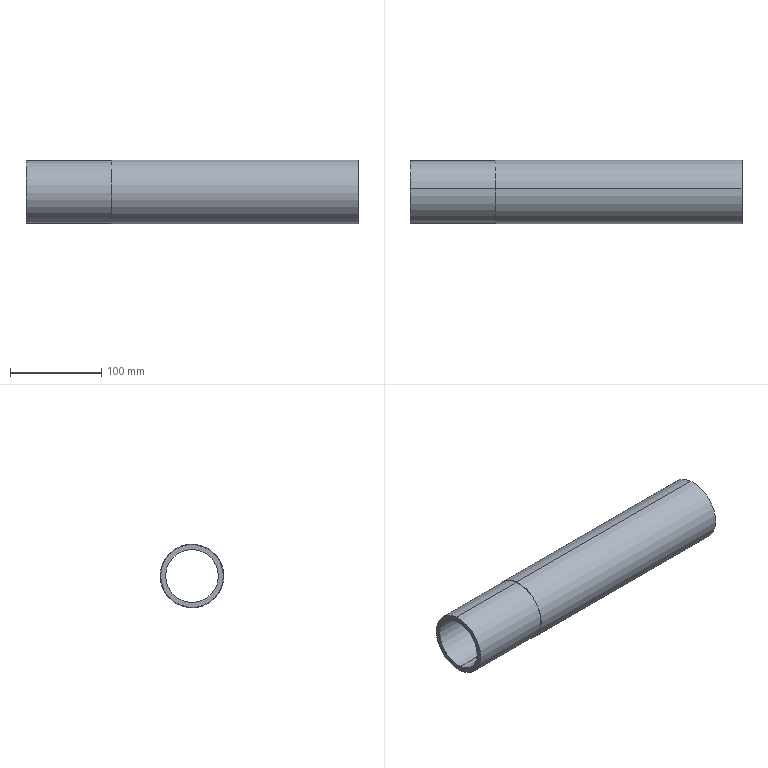Part | NX | features BREP 1 | 1 solid | 9 faces | box 364.46 x 70 x 70 mm | volume 429462 mm3 | cylinder 6 | plane 3 | commonest cylinder face diameters 58 x2 69 x2 70 x2
STEP:
#1=CARTESIAN_POINT('',(131.205,-2.874,-28.857));
#2=VERTEX_POINT('',#1);
#3=CARTESIAN_POINT('',(131.205,2.874,28.857));
#4=VERTEX_POINT('',#3);
#5=CARTESIAN_POINT('',(131.205,0.,0.));
#6=DIRECTION('',(-1.,0.,0.));
#7=DIRECTION('',(0.,0.09911,0.9951));
#8=AXIS2_PLACEMENT_3D('',#5,#6,#7);
#9=CIRCLE('',#8,29.);
#10=EDGE_CURVE('',#2,#4,#9,.T.);
#11=ORIENTED_EDGE('',*,*,#10,.T.);
#12=CARTESIAN_POINT('',(495.665,2.874,28.857));
#13=VERTEX_POINT('',#12);
#14=CARTESIAN_POINT('',(602.745,2.874,28.857));
#15=DIRECTION('',(1.,0.,0.));
#16=VECTOR('',#15,1000.);
#17=LINE('',#14,#16);
#18=EDGE_CURVE('',#13,#4,#17,.F.);
#19=ORIENTED_EDGE('',*,*,#18,.F.);
#20=CARTESIAN_POINT('',(495.665,-2.874,-28.857));
#21=VERTEX_POINT('',#20);
#22=CARTESIAN_POINT('',(495.665,0.,0.));
#23=DIRECTION('',(1.,0.,0.));
#24=DIRECTION('',(0.,0.,-1.));
#25=AXIS2_PLACEMENT_3D('',#22,#23,#24);
#26=CIRCLE('',#25,29.);
#27=EDGE_CURVE('',#13,#21,#26,.T.);
#28=ORIENTED_EDGE('',*,*,#27,.T.);
#29=CARTESIAN_POINT('',(602.745,-2.874,-28.857));
#30=DIRECTION('',(1.,0.,0.));
#31=VECTOR('',#30,1000.);
#32=LINE('',#29,#31);
#33=EDGE_CURVE('',#21,#2,#32,.F.);
#34=ORIENTED_EDGE('',*,*,#33,.T.);
#35=EDGE_LOOP('',(#11,#19,#28,#34));
#36=FACE_BOUND('',#35,.T.);
#37=CARTESIAN_POINT('',(602.745,0.,0.));
#38=DIRECTION('',(1.,0.,0.));
#39=DIRECTION('',(0.,0.09911,0.9951));
#40=AXIS2_PLACEMENT_3D('',#37,#38,#39);
#41=CYLINDRICAL_SURFACE('',#40,29.);
#42=ADVANCED_FACE('',(#36),#41,.F.);
#43=CARTESIAN_POINT('',(131.205,3.419,34.33));
#44=VERTEX_POINT('',#43);
#45=CARTESIAN_POINT('',(131.205,-3.419,-34.33));
#46=VERTEX_POINT('',#45);
#47=CARTESIAN_POINT('',(131.205,0.,0.));
#48=DIRECTION('',(-1.,0.,0.));
#49=DIRECTION('',(0.,0.09911,0.9951));
#50=AXIS2_PLACEMENT_3D('',#47,#48,#49);
#51=CIRCLE('',#50,34.5);
#52=EDGE_CURVE('',#44,#46,#51,.T.);
#53=ORIENTED_EDGE('',*,*,#52,.F.);
#54=CARTESIAN_POINT('',(224.745,3.419,34.33));
#55=VERTEX_POINT('',#54);
#56=CARTESIAN_POINT('',(131.205,3.419,34.33));
#57=DIRECTION('',(1.,0.,0.));
#58=VECTOR('',#57,1000.);
#59=LINE('',#56,#58);
#60=EDGE_CURVE('',#55,#44,#59,.F.);
#61=ORIENTED_EDGE('',*,*,#60,.F.);
#62=CARTESIAN_POINT('',(224.745,-3.419,-34.33));
#63=VERTEX_POINT('',#62);
#64=CARTESIAN_POINT('',(224.745,0.,0.));
#65=DIRECTION('',(-1.,0.,0.));
#66=DIRECTION('',(0.,0.09911,0.9951));
#67=AXIS2_PLACEMENT_3D('',#64,#65,#66);
#68=CIRCLE('',#67,34.5);
#69=EDGE_CURVE('',#55,#63,#68,.T.);
#70=ORIENTED_EDGE('',*,*,#69,.T.);
#71=CARTESIAN_POINT('',(131.205,-3.419,-34.33));
#72=DIRECTION('',(1.,0.,0.));
#73=VECTOR('',#72,1000.);
#74=LINE('',#71,#73);
#75=EDGE_CURVE('',#63,#46,#74,.F.);
#76=ORIENTED_EDGE('',*,*,#75,.T.);
#77=EDGE_LOOP('',(#53,#61,#70,#76));
#78=FACE_BOUND('',#77,.T.);
#79=CARTESIAN_POINT('',(131.205,0.,0.));
#80=DIRECTION('',(1.,0.,0.));
#81=DIRECTION('',(0.,0.09911,0.9951));
#82=AXIS2_PLACEMENT_3D('',#79,#80,#81);
#83=CYLINDRICAL_SURFACE('',#82,34.5);
#84=ADVANCED_FACE('',(#78),#83,.T.);
#85=CARTESIAN_POINT('',(224.745,-3.469,-34.828));
#86=VERTEX_POINT('',#85);
#87=CARTESIAN_POINT('',(224.745,3.469,34.828));
#88=VERTEX_POINT('',#87);
#89=CARTESIAN_POINT('',(224.745,0.,0.));
#90=DIRECTION('',(1.,0.,0.));
#91=DIRECTION('',(0.,-0.09911,-0.9951));
#92=AXIS2_PLACEMENT_3D('',#89,#90,#91);
#93=CIRCLE('',#92,35.);
#94=EDGE_CURVE('',#86,#88,#93,.T.);
#95=ORIENTED_EDGE('',*,*,#94,.T.);
#96=CARTESIAN_POINT('',(495.665,3.469,34.828));
#97=VERTEX_POINT('',#96);
#98=CARTESIAN_POINT('',(602.745,3.469,34.828));
#99=DIRECTION('',(1.,0.,0.));
#100=VECTOR('',#99,1000.);
#101=LINE('',#98,#100);
#102=EDGE_CURVE('',#97,#88,#101,.F.);
#103=ORIENTED_EDGE('',*,*,#102,.F.);
#104=CARTESIAN_POINT('',(495.665,-3.469,-34.828));
#105=VERTEX_POINT('',#104);
#106=CARTESIAN_POINT('',(495.665,0.,0.));
#107=DIRECTION('',(-1.,0.,0.));
#108=DIRECTION('',(0.,0.,-1.));
#109=AXIS2_PLACEMENT_3D('',#106,#107,#108);
#110=CIRCLE('',#109,35.);
#111=EDGE_CURVE('',#97,#105,#110,.T.);
#112=ORIENTED_EDGE('',*,*,#111,.T.);
#113=CARTESIAN_POINT('',(602.745,-3.469,-34.828));
#114=DIRECTION('',(1.,0.,0.));
#115=VECTOR('',#114,1000.);
#116=LINE('',#113,#115);
#117=EDGE_CURVE('',#105,#86,#116,.F.);
#118=ORIENTED_EDGE('',*,*,#117,.T.);
#119=EDGE_LOOP('',(#95,#103,#112,#118));
#120=FACE_BOUND('',#119,.T.);
#121=CARTESIAN_POINT('',(602.745,0.,0.));
#122=DIRECTION('',(1.,0.,0.));
#123=DIRECTION('',(0.,0.09911,0.9951));
#124=AXIS2_PLACEMENT_3D('',#121,#122,#123);
#125=CYLINDRICAL_SURFACE('',#124,35.);
#126=ADVANCED_FACE('',(#120),#125,.T.);
#127=CARTESIAN_POINT('',(495.665,0.,0.));
#128=DIRECTION('',(1.,0.,0.));
#129=DIRECTION('',(0.,0.,-1.));
#130=AXIS2_PLACEMENT_3D('',#127,#128,#129);
#131=CIRCLE('',#130,29.);
#132=EDGE_CURVE('',#21,#13,#131,.T.);
#133=ORIENTED_EDGE('',*,*,#132,.F.);
#134=ORIENTED_EDGE('',*,*,#27,.F.);
#135=EDGE_LOOP('',(#133,#134));
#136=FACE_BOUND('',#135,.T.);
#137=CARTESIAN_POINT('',(495.665,0.,0.));
#138=DIRECTION('',(-1.,0.,0.));
#139=DIRECTION('',(0.,0.,-1.));
#140=AXIS2_PLACEMENT_3D('',#137,#138,#139);
#141=CIRCLE('',#140,35.);
#142=EDGE_CURVE('',#105,#97,#141,.T.);
#143=ORIENTED_EDGE('',*,*,#142,.F.);
#144=ORIENTED_EDGE('',*,*,#111,.F.);
#145=EDGE_LOOP('',(#143,#144));
#146=FACE_BOUND('',#145,.T.);
#147=CARTESIAN_POINT('',(495.665,-40.903,-44.627));
#148=DIRECTION('',(1.,0.,0.));
#149=DIRECTION('',(0.,0.,1.));
#150=AXIS2_PLACEMENT_3D('',#147,#148,#149);
#151=PLANE('',#150);
#152=ADVANCED_FACE('',(#136,#146),#151,.T.);
#153=CARTESIAN_POINT('',(224.745,0.,0.));
#154=DIRECTION('',(-1.,0.,0.));
#155=DIRECTION('',(0.,0.09911,0.9951));
#156=AXIS2_PLACEMENT_3D('',#153,#154,#155);
#157=CIRCLE('',#156,34.5);
#158=EDGE_CURVE('',#63,#55,#157,.T.);
#159=ORIENTED_EDGE('',*,*,#158,.F.);
#160=ORIENTED_EDGE('',*,*,#69,.F.);
#161=EDGE_LOOP('',(#159,#160));
#162=FACE_BOUND('',#161,.T.);
#163=ORIENTED_EDGE('',*,*,#94,.F.);
#164=CARTESIAN_POINT('',(224.745,0.,0.));
#165=DIRECTION('',(1.,0.,0.));
#166=DIRECTION('',(0.,-0.09911,-0.9951));
#167=AXIS2_PLACEMENT_3D('',#164,#165,#166);
#168=CIRCLE('',#167,35.);
#169=EDGE_CURVE('',#88,#86,#168,.T.);
#170=ORIENTED_EDGE('',*,*,#169,.F.);
#171=EDGE_LOOP('',(#163,#170));
#172=FACE_BOUND('',#171,.T.);
#173=CARTESIAN_POINT('',(224.745,0.,0.));
#174=DIRECTION('',(1.,0.,0.));
#175=DIRECTION('',(0.,0.09911,0.9951));
#176=AXIS2_PLACEMENT_3D('',#173,#174,#175);
#177=PLANE('',#176);
#178=ADVANCED_FACE('',(#162,#172),#177,.F.);
#179=ORIENTED_EDGE('',*,*,#102,.T.);
#180=ORIENTED_EDGE('',*,*,#169,.T.);
#181=ORIENTED_EDGE('',*,*,#117,.F.);
#182=ORIENTED_EDGE('',*,*,#142,.T.);
#183=EDGE_LOOP('',(#179,#180,#181,#182));
#184=FACE_BOUND('',#183,.T.);
#185=CARTESIAN_POINT('',(602.745,0.,0.));
#186=DIRECTION('',(1.,0.,0.));
#187=DIRECTION('',(0.,0.09911,0.9951));
#188=AXIS2_PLACEMENT_3D('',#185,#186,#187);
#189=CYLINDRICAL_SURFACE('',#188,35.);
#190=ADVANCED_FACE('',(#184),#189,.T.);
#191=ORIENTED_EDGE('',*,*,#60,.T.);
#192=CARTESIAN_POINT('',(131.205,0.,0.));
#193=DIRECTION('',(-1.,0.,0.));
#194=DIRECTION('',(0.,0.09911,0.9951));
#195=AXIS2_PLACEMENT_3D('',#192,#193,#194);
#196=CIRCLE('',#195,34.5);
#197=EDGE_CURVE('',#46,#44,#196,.T.);
#198=ORIENTED_EDGE('',*,*,#197,.F.);
#199=ORIENTED_EDGE('',*,*,#75,.F.);
#200=ORIENTED_EDGE('',*,*,#158,.T.);
#201=EDGE_LOOP('',(#191,#198,#199,#200));
#202=FACE_BOUND('',#201,.T.);
#203=CARTESIAN_POINT('',(131.205,0.,0.));
#204=DIRECTION('',(1.,0.,0.));
#205=DIRECTION('',(0.,0.09911,0.9951));
#206=AXIS2_PLACEMENT_3D('',#203,#204,#205);
#207=CYLINDRICAL_SURFACE('',#206,34.5);
#208=ADVANCED_FACE('',(#202),#207,.T.);
#209=ORIENTED_EDGE('',*,*,#10,.F.);
#210=CARTESIAN_POINT('',(131.205,0.,0.));
#211=DIRECTION('',(-1.,0.,0.));
#212=DIRECTION('',(0.,0.09911,0.9951));
#213=AXIS2_PLACEMENT_3D('',#210,#211,#212);
#214=CIRCLE('',#213,29.);
#215=EDGE_CURVE('',#4,#2,#214,.T.);
#216=ORIENTED_EDGE('',*,*,#215,.F.);
#217=EDGE_LOOP('',(#209,#216));
#218=FACE_BOUND('',#217,.T.);
#219=ORIENTED_EDGE('',*,*,#197,.T.);
#220=ORIENTED_EDGE('',*,*,#52,.T.);
#221=EDGE_LOOP('',(#219,#220));
#222=FACE_BOUND('',#221,.T.);
#223=CARTESIAN_POINT('',(131.205,0.,0.));
#224=DIRECTION('',(-1.,0.,0.));
#225=DIRECTION('',(0.,-0.09911,-0.9951));
#226=AXIS2_PLACEMENT_3D('',#223,#224,#225);
#227=PLANE('',#226);
#228=ADVANCED_FACE('',(#218,#222),#227,.T.);
#229=ORIENTED_EDGE('',*,*,#18,.T.);
#230=ORIENTED_EDGE('',*,*,#215,.T.);
#231=ORIENTED_EDGE('',*,*,#33,.F.);
#232=ORIENTED_EDGE('',*,*,#132,.T.);
#233=EDGE_LOOP('',(#229,#230,#231,#232));
#234=FACE_BOUND('',#233,.T.);
#235=CARTESIAN_POINT('',(602.745,0.,0.));
#236=DIRECTION('',(1.,0.,0.));
#237=DIRECTION('',(0.,0.09911,0.9951));
#238=AXIS2_PLACEMENT_3D('',#235,#236,#237);
#239=CYLINDRICAL_SURFACE('',#238,29.);
#240=ADVANCED_FACE('',(#234),#239,.F.);
#241=CLOSED_SHELL('',(#42,#84,#126,#152,#178,#190,#208,#228,#240));
#242=MANIFOLD_SOLID_BREP('',#241);
#243=(LENGTH_UNIT()NAMED_UNIT(*)SI_UNIT(.MILLI.,.METRE.));
#244=UNCERTAINTY_MEASURE_WITH_UNIT(LENGTH_MEASURE(0.00001),#243,'','');
#245=(NAMED_UNIT(*)PLANE_ANGLE_UNIT()SI_UNIT($,.RADIAN.));
#246=(NAMED_UNIT(*)SI_UNIT($,.STERADIAN.)SOLID_ANGLE_UNIT());
#247=(GEOMETRIC_REPRESENTATION_CONTEXT(3)GLOBAL_UNCERTAINTY_ASSIGNED_CONTEXT((#244))GLOBAL_UNIT_ASSIGNED_CONTEXT((#243,#245,#246))REPRESENTATION_CONTEXT('',''));
#248=ADVANCED_BREP_SHAPE_REPRESENTATION('',(#242),#247);